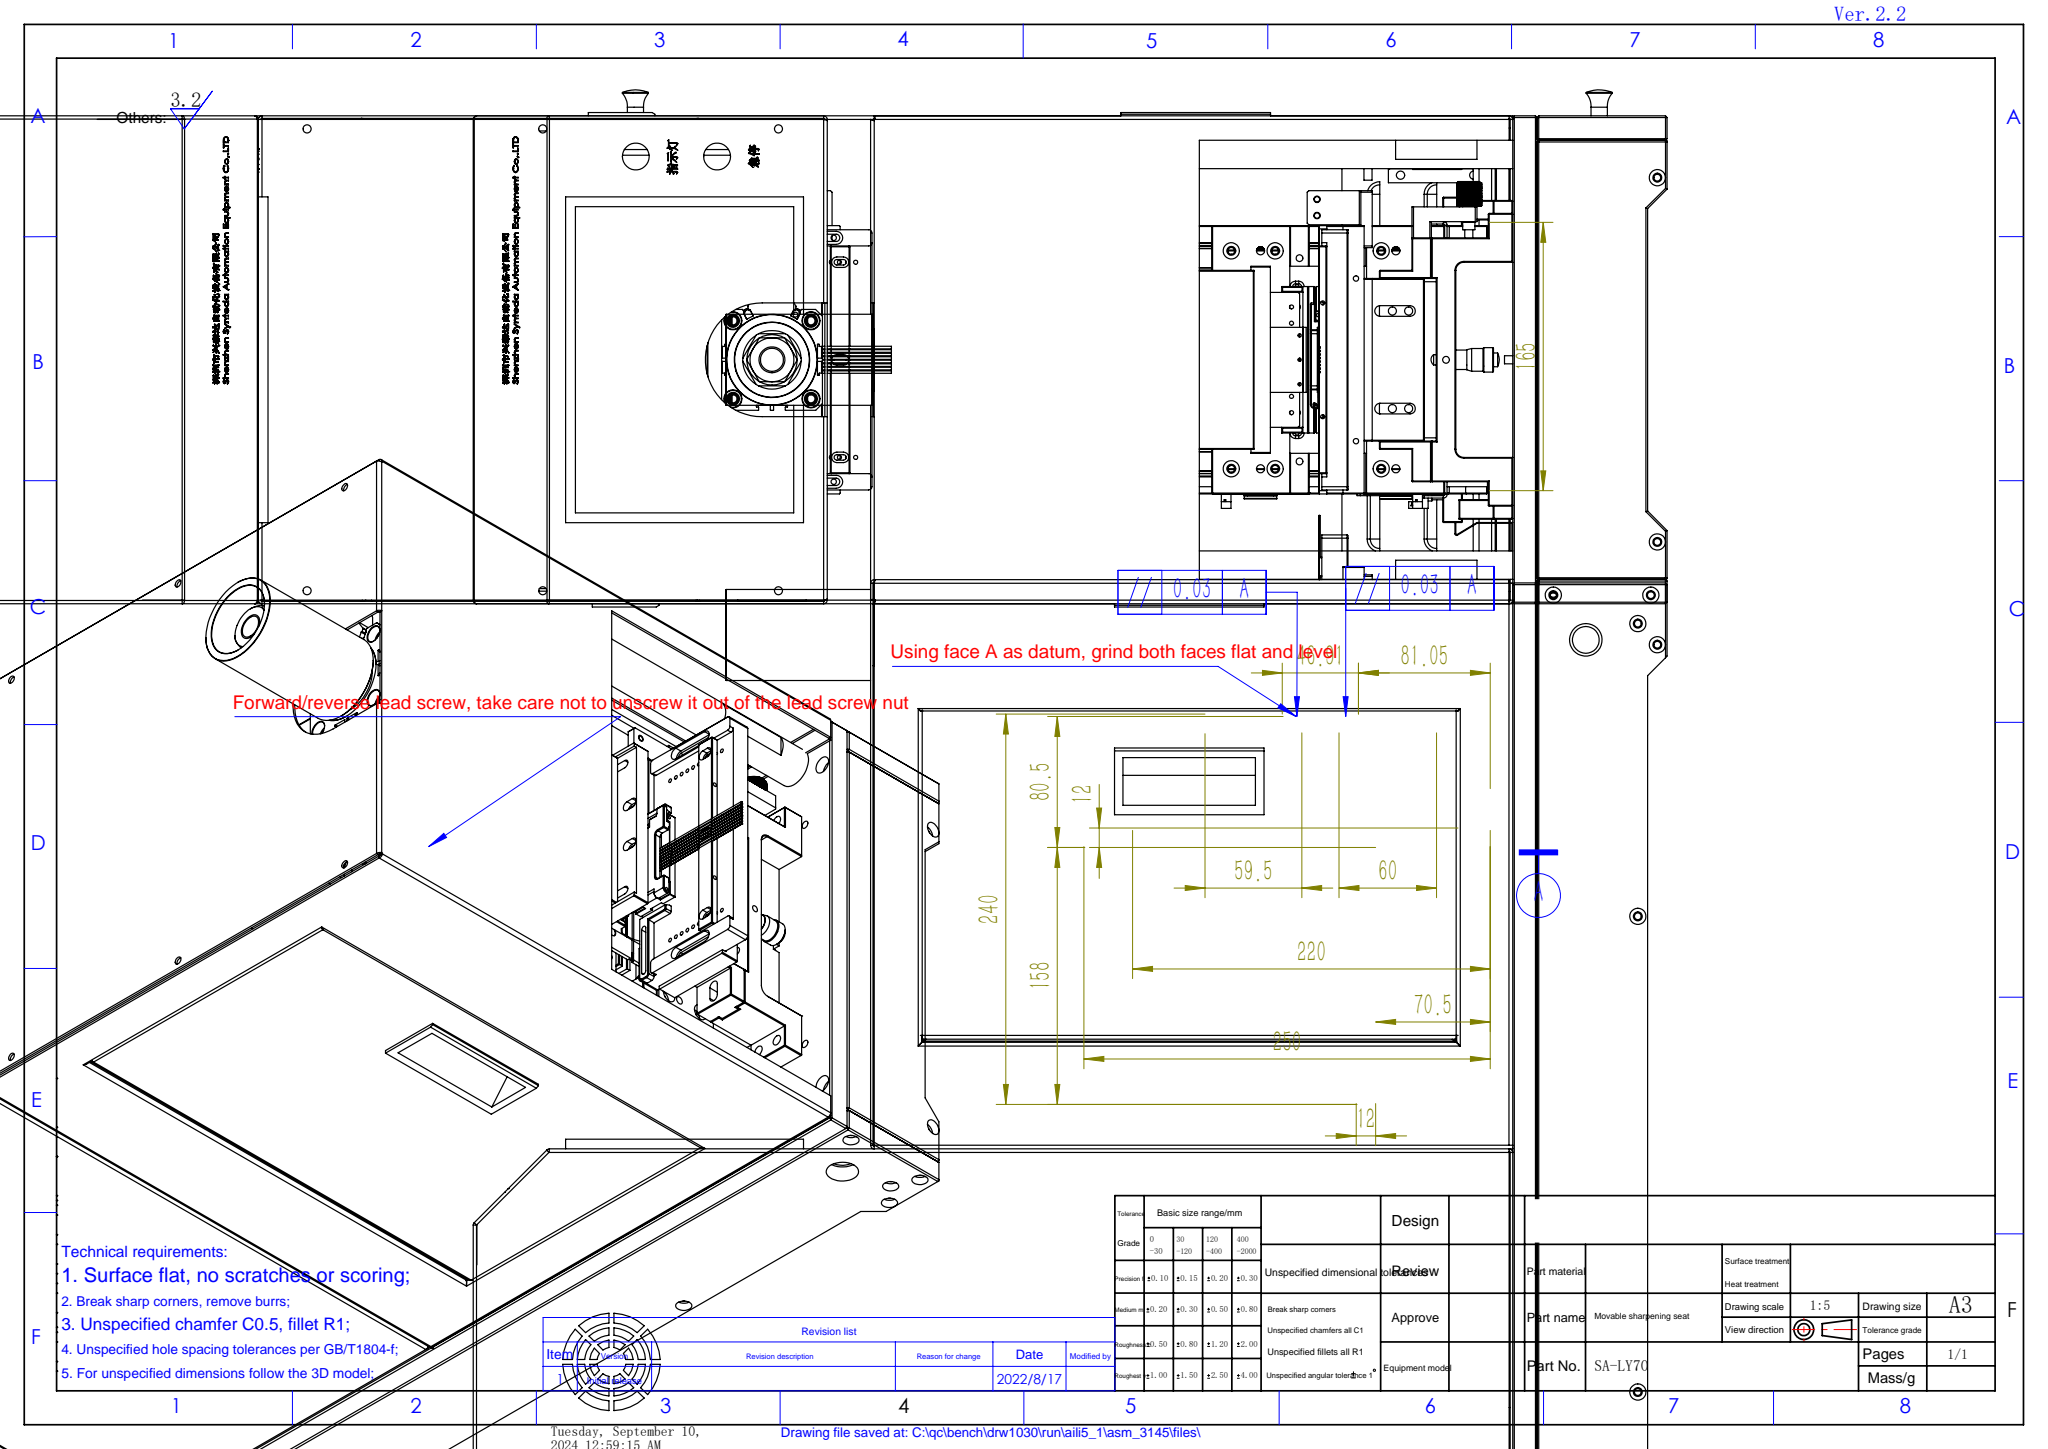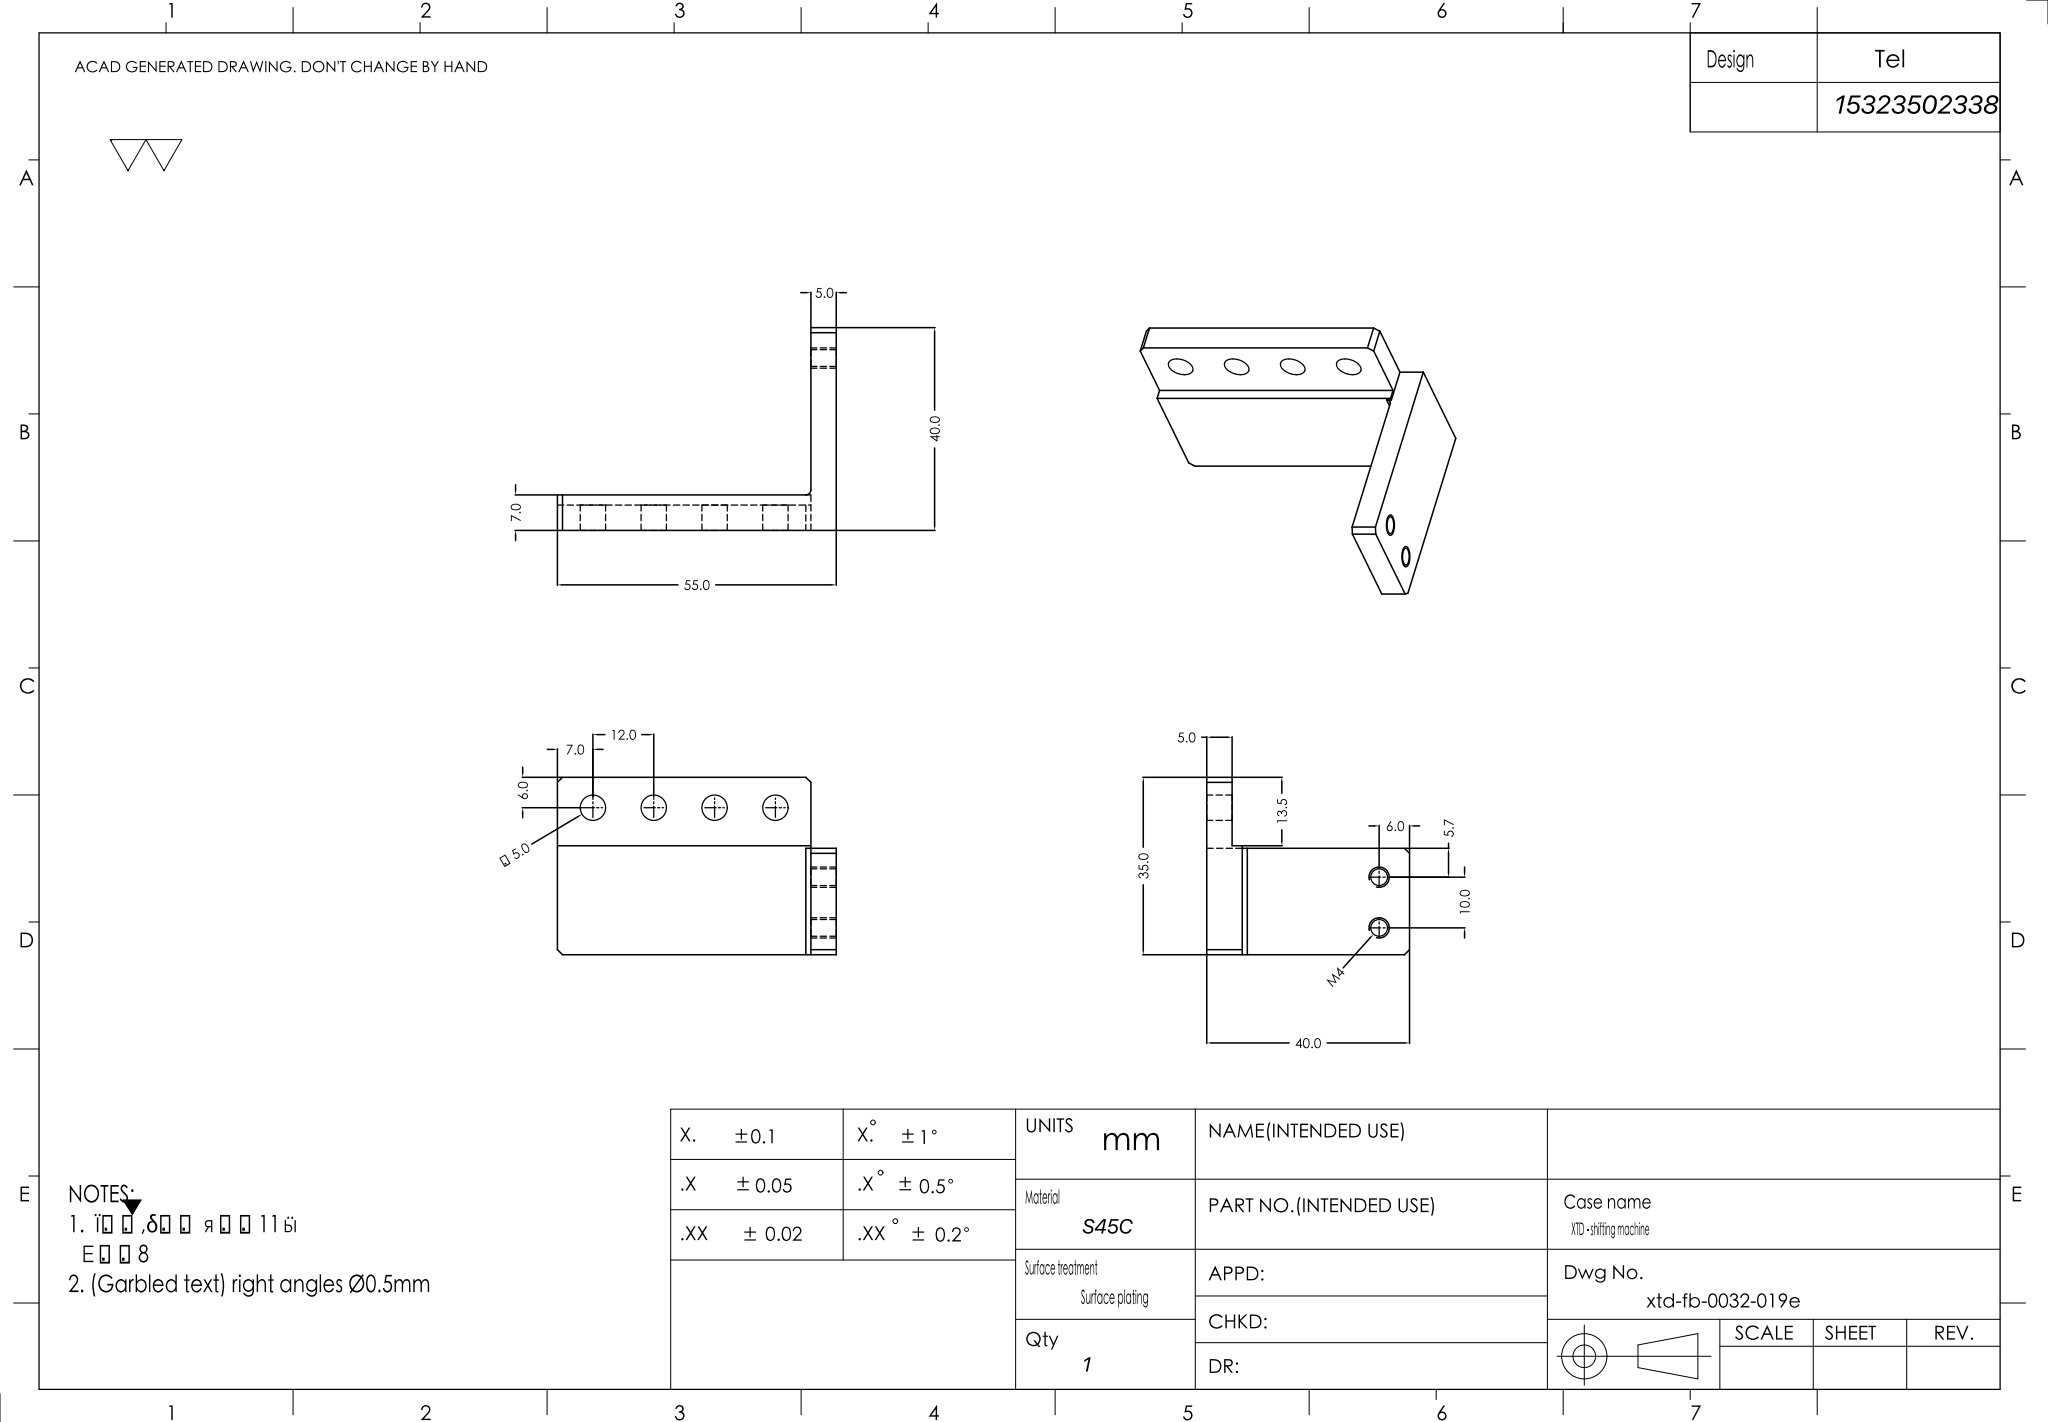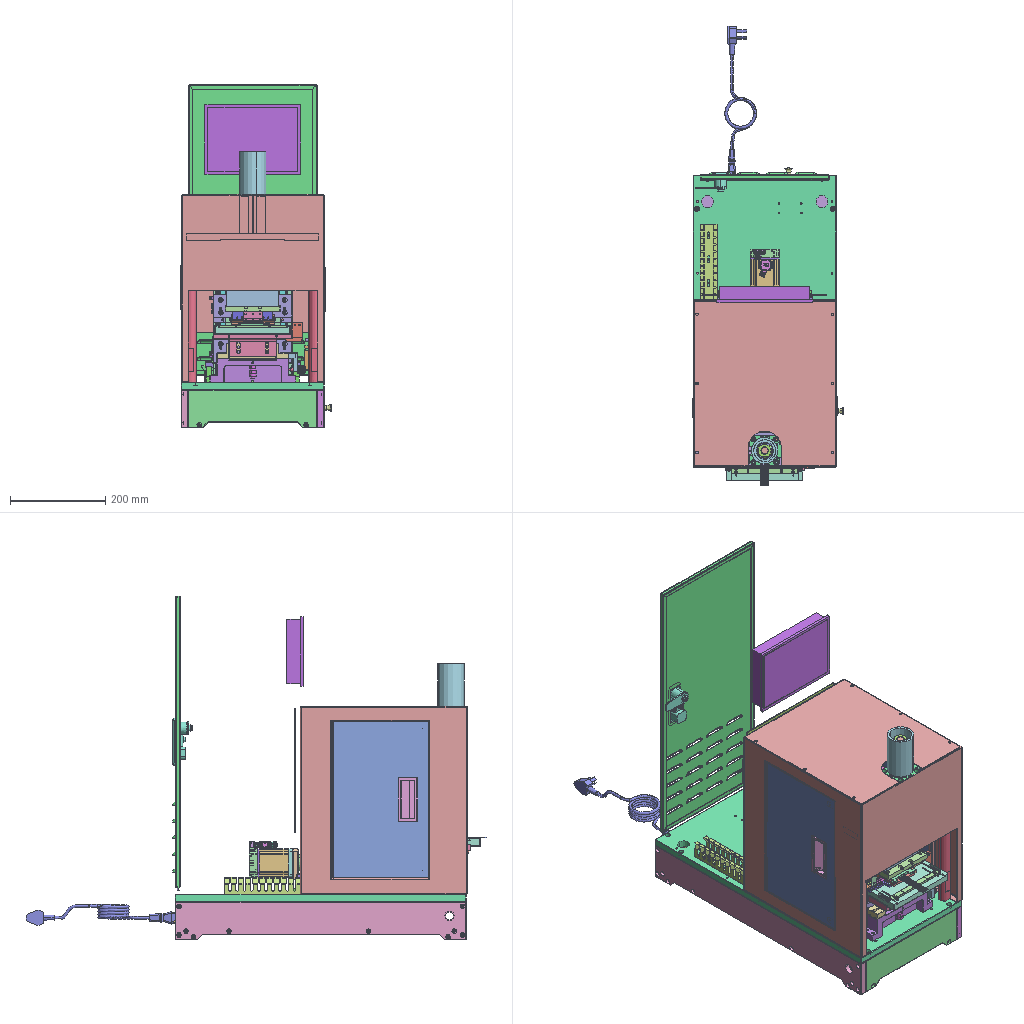Assembly | SolidWorks | 205 different items | 269 placed | box 318 x 965 x 720 mm
Parts list (item | name | quantity | parent item | size | volume | features):
1 | 0014 | x1 | - | - | - | -
2 | (subassembly) | x1 | in 17 | 12 x 43 x 43 mm | 7993 mm3 | -
3 | (subassembly) | x1 | in 17 | 110 x 14 x 40 mm | 34476 mm3 | -
4 | (subassembly) | x1 | - | 356.977 x 304 x 446.493 mm | 211386 mm3 | features ReferencePattern 2, InContextFeatHolder 1, MirrorCompFeat 1
5 | (subassembly) | x1 | - | 625.233 x 304 x 617.993 mm | 1412506 mm3 | features CompositeCurve 2, LocalLPattern 2, ReferencePattern 2
6 | (subassembly) | x1 | - | - | 1320917 mm3 | -
7 | (subassembly) | x1 | in 16 | 168.001 x 57 x 60 mm | 203187 mm3 | -
8 | (subassembly) | x1 | in 16 | 170.787 x 57.213 x 123 mm | 228547 mm3 | -
9 | (subassembly) | x1 | - | - | 1768279 mm3 | -
10 | (subassembly) | x1 | - | 316 x 923.1 x 130.5 mm | 5362274 mm3 | -
11 | (subassembly) | x1 | in 6 | 20 x 43 x 70 mm | 38437 mm3 | -
12 | (subassembly) | x1 | in 23 | - | - | -
13 | (subassembly) | x1 | in 6 | 35.5 x 43 x 70 mm | 61355 mm3 | -
14 | (subassembly) | x1 | in 17 | 150 x 40 x 36.569 mm | 33298 mm3 | -
15 | (subassembly) | x1 | in 6 | 150 x 39.987 x 40 mm | 33298 mm3 | -
16 | (subassembly) | x1 | - | - | 1570886 mm3 | -
17 | (subassembly) | x1 | - | - | 638711 mm3 | features CompositeCurve 1
18 | (subassembly) | x1 | in 16 | 40 x 213 x 40 mm | 59084 mm3 | -
19 | (subassembly) | x1 | in 16 | - | - | -
20 | (subassembly) | x1 | in 6 | 60 x 74.1 x 121 mm | 300230 mm3 | -
21 | (subassembly) | x1 | in 23 | - | - | -
22 | (subassembly) | x1 | in 12 | - | - | -
23 | (subassembly) | x1 | in 9 | 164.031 x 194.596 x 81.627 mm | 348427 mm3 | -
24 | (subassembly) | x1 | in 9 | 47 x 35.487 x 115 mm | 62999 mm3 | -
25 | (subassembly) | x2 | in 16 | 34 x 24 x 220 mm | 96136 mm3 | -
26 | (subassembly) | x2 | in 6 | 34 x 160 x 24 mm | 68410 mm3 | -
27 | (subassembly) | x2 | in 16, 17 | 35 x 52 x 52 mm | 28520 mm3 | -
28 | ATH-B0001 | x1 | - | - | - | -
29 | BML01-M6-L20 | x1 | - | - | - | -
30 | - | x1 | in 22 | - | - | features RefSurface 1
31 | - | x1 | in 17 | 70 x 72.5 x 10 mm | 34993 mm3 | features HoleWzd 3, Chamfer 2, Cut 2, Extrusion 1
32 | - | x1 | in 17 | 70 x 55 x 10 mm | 17124 mm3 | features Chamfer 2, Cut 2, HoleWzd 2, Extrusion 1, ICE 1
33 | - | x1 | in 17 | 70 x 55 x 10 mm | 20191 mm3 | features Chamfer 2, Cut 2, HoleWzd 2, Extrusion 1, ICE 1
34 | - | x1 | in 17 | 46 x 48 x 30 mm | 41518 mm3 | features HoleWzd 5, Chamfer 1, Cut 1, Extrusion 1, ICE 1
35 | - | x1 | in 17 | 76 x 68.5 x 10 mm | 24767 mm3 | features HoleWzd 4, Cut 3, Fillet 2, Chamfer 1, Extrusion 1, ICE 1
36 | - | x1 | in 17 | 60 x 76 x 14 mm | 29747 mm3 | features Cut 2, HoleWzd 2, Chamfer 1, Extrusion 1, Fillet 1, ICE 1
37 | - | x1 | in 17 | 120 x 35 x 10 mm | 16270 mm3 | features BaseBody 1
38 | - | x1 | in 10 | 235 x 120 x 40 mm | 81570 mm3 | features EdgeFlange 1, FlatPattern 1, HoleWzd 1, SMBaseFlange 1, SheetMetal 1
39 | - | x1 | in 10 | 40 x 100 x 120 mm | 42493 mm3 | features SMWeldBead 4, EdgeFlange 1, FlatPattern 1, HoleWzd 1, SMBaseFlange 1, SheetMetal 1
40 | - | x1 | in 8 | 170.003 x 76.5 x 17.003 mm | 25360 mm3 | features EdgeFlange 4, SMBaseFlange 2, Chamfer 1, FlatPattern 1, HoleWzd 1, SheetMetal 1
41 | - | x1 | in 22 | - | - | features RefSurface 1
42 | - | x2 | in 7, 8 | 20 x 36.964 x 3 mm | 709.216 mm3 | features EdgeFlange 2, Fillet 1, FlatPattern 1, HoleWzd 1, SMBaseFlange 1, SheetMetal 1
43 | - | x1 | in 16 | 20 x 36.464 x 3 mm | 699.216 mm3 | features EdgeFlange 2, Fillet 1, FlatPattern 1, HoleWzd 1, SMBaseFlange 1, SheetMetal 1
44 | - | x1 | in 17 | 20 x 36.5 x 25.2 mm | 1153 mm3 | features EdgeFlange 2, Fillet 1, FlatPattern 1, HoleWzd 1, SMBaseFlange 1, SheetMetal 1
45 | - | x1 | in 6 | 160 x 9 x 6 mm | 4968 mm3 | features BaseBody 1, Cut 1, HoleWzd 1, ICE 1, MoveFace 1
46 | - | x1 | in 17 | 105 x 9 x 6 mm | 3236 mm3 | features ICE 2, BaseBody 1, Cut 1, HoleWzd 1, MoveFace 1
47 | - | x1 | in 16 | 220 x 9 x 6 mm | 6858 mm3 | features BaseBody 1, Cut 1, HoleWzd 1, ICE 1, MoveFace 1
48 | - | x1 | - | 30 x 19 x 40 mm | 12917 mm3 | features ICE 2, Chamfer 1, Extrusion 1, HoleWzd 1
49 | - | x1 | - | 56 x 90 x 56 mm | 77215 mm3 | features Chamfer 1, Extrusion 1, ICE 1
50 | - | x1 | - | 35 x 35 x 2 mm | 1232 mm3 | features Extrusion 1
51 | - | x1 | in 9 | 170 x 62 x 71.5 mm | 267417 mm3 | features BaseBody 6
52 | - | x1 | in 22 | - | - | features RefSurface 1
53 | - | x1 | - | - | 2705 mm3 | features BaseBody 1
54 | - | x1 | in 9 | 8.4 x 18.475 x 16 mm | 1325 mm3 | features BaseBody 1
55 | - | x1 | in 9 | 17 x 19.6 x 45 mm | 6217 mm3 | features BaseBody 1
56 | - | x1 | in 23 | 55 x 50 x 165 mm | 141740 mm3 | features HoleWzd 5, ICE 2, Chamfer 1, Extrusion 1
57 | - | x1 | in 23 | - | - | features RefSurface 2, BaseBody 1
58 | - | x1 | in 24 | 7.5 x 20 x 90 mm | 7139 mm3 | features Chamfer 1, Extrusion 1, Fillet 1, HoleWzd 1, ICE 1
59 | - | x1 | in 23 | 140 x 12 x 5 mm | 7481 mm3 | features HoleWzd 2, Chamfer 1, Extrusion 1
60 | - | x2 | - | 115 x 2.5 x 23 mm | 5943 mm3 | features ICE 2, Extrusion 1, HoleWzd 1
61 | - | x1 | in 23 | 90 x 32.1 x 7 mm | 12925 mm3 | features Chamfer 3, Fillet 2, Extrusion 1, HoleWzd 1, ICE 1
62 | - | x1 | in 22 | - | - | features RefSurface 1
63 | - | x1 | in 24 | 40 x 7 x 21.5 mm | 5238 mm3 | features HoleWzd 2, Cut 1, Extrusion 1
64 | - | x1 | in 24 | 83 x 28 x 6 mm | 13498 mm3 | features HoleWzd 2, Chamfer 1, Extrusion 1
65 | - | x1 | in 24 | 40 x 7 x 6 mm | 1162 mm3 | features ICE 2, Extrusion 1
66 | - | x1 | in 24 | 115 x 12 x 37 mm | 35962 mm3 | features ICE 8, Cut 4, HoleWzd 4, Chamfer 1, Extrusion 1
67 | - | x2 | in 23 | 50 x 6 x 9 mm | 2366 mm3 | features Chamfer 1, Extrusion 1, HoleWzd 1
68 | - | x1 | in 23 | 90 x 10 x 5 mm | 4179 mm3 | features Chamfer 2, Extrusion 1, HoleWzd 1
69 | - | x1 | in 23 | 160 x 80 x 16 mm | 159297 mm3 | features ICE 8, HoleWzd 5, Chamfer 4, Extrusion 1, Fillet 1, LPattern 1
70 | - | x1 | in 23 | 47.5 x 23 x 5 mm | 1583 mm3 | features Fillet 2, Chamfer 1, Extrusion 1, HoleWzd 1, ICE 1
71 | - | x1 | in 23 | 47.5 x 23 x 5 mm | 1583 mm3 | features Fillet 2, Chamfer 1, Extrusion 1, HoleWzd 1, ICE 1
72 | - | x2 | in 2, 11 | 7 x 22 x 22 mm | 1819 mm3 | features BaseBody 1
73 | - | x1 | in 22 | - | - | features RefSurface 1
74 | - | x2 | in 14, 15 | 150 x 12 x 12 mm | 13946 mm3 | features BaseBody 1
75 | - | x2 | in 27 | 52 x 52 x 23 mm | 13989 mm3 | features BaseBody 1
76 | - | x2 | in 27 | 6.1 x 52 x 52 mm | 4618 mm3 | features BaseBody 1
77 | - | x2 | in 27 | 16 x 26 x 26 mm | 6727 mm3 | features BaseBody 1
78 | - | x4 | in 27 | 3 x 21 x 21 mm | 508.938 mm3 | features BaseBody 1
79 | - | x1 | in 2 | 43 x 43 x 12 mm | 6140 mm3 | features BaseBody 1
80 | - | x1 | in 11 | 70 x 43 x 20 mm | 36584 mm3 | features BaseBody 1
81 | - | x1 | in 13 | 24 x 43 x 70 mm | 47260 mm3 | features BaseBody 1
82 | - | x1 | in 13 | 8.1 x 34 x 34 mm | 4182 mm3 | features BaseBody 1
83 | - | x1 | in 13 | 16 x 26 x 26 mm | 6727 mm3 | features BaseBody 1
84 | - | x1 | in 22 | - | - | features RefSurface 1
85 | - | x2 | in 13 | 3 x 21 x 21 mm | 508.938 mm3 | features BaseBody 1
86 | - | x2 | in 27 | 19 x 19 x 8 mm | 1253 mm3 | features BaseBody 1
87 | - | x1 | in 13 | 19 x 19 x 8 mm | 1253 mm3 | features BaseBody 1
88 | - | x4 | in 27 | 14.4 x 14.4 x 5.5 mm | 457.404 mm3 | features BaseBody 1
89 | - | x2 | in 13 | 14.4 x 14.4 x 5.5 mm | 457.404 mm3 | features BaseBody 1
90 | - | x2 | in 2, 11 | 9.8 x 12 x 0.8 mm | 33.948 mm3 | features BaseBody 1
91 | - | x2 | in 10 | 16 x 22 x 16 mm | 1745 mm3 | features BaseBody 1
92 | - | x2 | in 17 | 10.392 x 19.5 x 9.5 mm | 848.731 mm3 | features BaseBody 1
93 | - | x1 | in 10 | 66.481 x 44.258 x 325.5 mm | 63656 mm3 | features MirrorStock 1
94 | - | x1 | in 10 | 35 x 35.5 x 353 mm | 17858 mm3 | features BaseBody 1, ICE 1
95 | - | x1 | in 22 | - | - | features RefSurface 1
96 | - | x2 | in 5 | 23.155 x 48.5 x 92 mm | 9910 mm3 | features BaseBody 1
97 | - | x1 | - | - | - | features RefSurface 1
98 | - | x1 | - | - | - | features RefSurface 1
99 | - | x1 | - | - | - | features RefSurface 1
100 | - | x1 | - | - | - | features RefSurface 1
101 | - | x1 | - | - | - | features RefSurface 1
102 | - | x3 | in 14, 15, 18 | 40 x 40 x 32 mm | 19352 mm3 | features BaseBody 1
103 | - | x1 | in 18 | 40 x 40 x 32 mm | 19352 mm3 | features BaseBody 1
104 | - | x1 | in 18 | 12 x 213 x 12 mm | 20380 mm3 | features BaseBody 1
105 | - | x1 | in 5 | 260 x 260 x 2 mm | 135000 mm3 | features Extrusion 1, Fillet 1, HoleWzd 1
106 | - | x1 | in 22 | - | - | features RefSurface 1
107 | - | x1 | in 10 | 51 x 50 x 32.3 mm | 28039 mm3 | features MirrorStock 1
108 | - | x1 | - | - | - | features RefSurface 1
109 | - | x1 | - | - | - | features RefSurface 1
110 | - | x1 | - | - | - | features RefSurface 1
111 | - | x1 | in 22 | - | - | features RefSurface 1
112 | - | x1 | in 22 | - | - | features RefSurface 1
113 | - | x1 | in 12 | - | - | features RefSurface 1
114 | - | x1 | in 22 | - | - | features RefSurface 1
115 | - | x1 | in 22 | - | - | features RefSurface 1
116 | - | x1 | in 22 | - | - | features RefSurface 1
117 | - | x1 | in 22 | - | - | features RefSurface 1
118 | - | x1 | in 22 | - | - | features RefSurface 1
119 | - | x1 | in 22 | - | - | features RefSurface 1
120 | - | x1 | in 22 | - | - | features RefSurface 1
121 | - | x1 | in 22 | - | - | features RefSurface 1
122 | - | x1 | in 22 | - | - | features RefSurface 1
123 | - | x1 | in 22 | - | - | features RefSurface 1
124 | - | x1 | in 22 | - | - | features RefSurface 1
125 | - | x1 | in 22 | - | - | features RefSurface 1
126 | - | x1 | in 22 | - | - | features RefSurface 1
127 | - | x1 | in 22 | - | - | features RefSurface 1
128 | - | x1 | in 22 | - | - | features RefSurface 1
129 | - | x1 | in 22 | - | - | features RefSurface 1
130 | - | x1 | in 17 | - | 141786 mm3 | features BaseBody 32
131 | - | x1 | - | - | - | features RefSurface 1
132 | - | x1 | - | - | - | features RefSurface 1
133 | - | x1 | - | - | - | features RefSurface 1
134 | - | x1 | - | - | - | features RefSurface 1
135 | - | x1 | in 22 | - | - | features RefSurface 1
136 | - | x1 | - | - | - | features RefSurface 1
137 | - | x4 | in 5 | 8 x 8 x 2 mm | 76.985 mm3 | features BaseBody 1
138 | - | x2 | in 6, 16 | 35 x 34 x 34 mm | 22881 mm3 | features BaseBody 1
139 | - | x1 | in 17 | 35 x 34 x 34 mm | 23327 mm3 | features BaseBody 1
140 | - | x9 | in 6, 16, 17 | 14.9 x 24.3 x 11.7 mm | 940.552 mm3 | features BaseBody 1
141 | - | x2 | in 26 | 15 x 12.5 x 160 mm | 25521 mm3 | features BaseBody 1
142 | - | x2 | in 25 | 15 x 12.5 x 220 mm | 34973 mm3 | features BaseBody 1, HoleWzd 1, MoveFace 1
143 | - | x1 | in 5 | 17.6 x 9 x 84 mm | 4996 mm3 | features BaseBody 2
144 | - | x1 | in 16 | 52 x 52 x 15 mm | 13321 mm3 | features BaseBody 1
145 | - | x4 | in 26 | 34 x 19.5 x 41.1 mm | 21445 mm3 | features BaseBody 1
146 | - | x1 | in 22 | - | - | features RefSurface 1
147 | - | x1 | in 5 | 395 x 300 x 350 mm | 661640 mm3 | features ICE 5, EdgeFlange 4, Cut 1, Fillet 1, FlatPattern 1, HoleWzd 1, LPattern 1, MirrorPattern 1, SMBaseFlange 1, SheetMetal 1
148 | - | x2 | in 5 | 333 x 204 x 10 mm | 124436 mm3 | features EdgeFlange 2, ICE 2, Cut 1, Fillet 1, FlatPattern 1, HoleWzd 1, SMBaseFlange 1, SheetMetal 1
149 | - | x4 | in 25 | 34 x 19.5 x 57.8 mm | 30582 mm3 | features BaseBody 1
150 | - | x1 | in 5 | 69.5 x 40 x 100 mm | 51575 mm3 | features BaseBody 1
151 | - | x1 | in 5 | - | - | -
152 | - | x1 | in 5 | 610.973 x 271.523 x 15.997 mm | 290304 mm3 | features EdgeFlange 2, Cut 1, FlatPattern 1, FormToolInstance 1, LPattern 1, SMBaseFlange 1, SheetMetal 1
153 | - | x1 | in 3 | 40 x 10.6 x 46.1 mm | 13496 mm3 | features BaseBody 1
154 | - | x1 | in 3 | 24 x 8.5 x 110 mm | 20980 mm3 | features BaseBody 1
155 | - | x1 | in 9 | 42 x 15 x 15 mm | 4392 mm3 | features BaseBody 1
156 | - | x1 | in 19 | - | - | features BaseBody 21, RefSurface 11
157 | - | x1 | in 22 | - | - | features RefSurface 1
158 | - | x1 | in 20 | 60 x 74.1 x 121 mm | 300230 mm3 | features BaseBody 24
159 | - | x1 | - | 200.3 x 146.3 x 34 mm | 870408 mm3 | features ICE 2, Extrusion 1
160 | - | x1 | - | - | - | features RefSurface 1
161 | - | x2 | in 9 | 37.5 x 47.5 x 18 mm | 8206 mm3 | features BaseBody 1
162 | - | x2 | in 19, 20 | - | - | -
163 | - | x2 | in 19, 20 | - | - | -
164 | - | x2 | in 19, 20 | - | - | -
165 | - | x1 | in 9 | 296 x 62 x 15 mm | 226499 mm3 | features HoleWzd 3, Chamfer 2, Cut 2, Extrusion 1
166 | - | x1 | in 9 | 135 x 100 x 27 mm | 173554 mm3 | features HoleWzd 2, ICE 2, Chamfer 1, Cut 1, Extrusion 1, Fillet 1
167 | - | x1 | in 9 | 110 x 90 x 15 mm | 144771 mm3 | features Cut 2, Chamfer 1, Extrusion 1, HoleWzd 1
168 | - | x1 | in 22 | - | - | features RefSurface 1
169 | - | x2 | in 9 | 10 x 100 x 20 mm | 18869 mm3 | features Chamfer 1, Extrusion 1, HoleWzd 1
170 | - | x2 | in 9 | 25 x 25 x 300 mm | 142022 mm3 | features Chamfer 1, Extrusion 1, HoleWzd 1, ICE 1, MirrorPattern 1
171 | - | x1 | in 9 | 180 x 30 x 50 mm | 139054 mm3 | features Cut 4, HoleWzd 4, ICE 2, Chamfer 1, Extrusion 1, Fillet 1
172 | - | x1 | in 9 | 150 x 35 x 30 mm | 55419 mm3 | features ICE 4, Chamfer 1, Extrusion 1, HoleWzd 1, LPattern 1
173 | - | x1 | in 10 | 270 x 80 x 15 mm | 285008 mm3 | features HoleWzd 3, Chamfer 2, Cut 1, Extrusion 1, MirrorPattern 1
174 | - | x1 | in 10 | 270 x 80 x 15 mm | 180697 mm3 | features Cut 4, HoleWzd 4, Chamfer 2, ICE 2, Extrusion 1, Fillet 1, MirrorPattern 1
175 | - | x1 | in 10 | 200 x 270 x 12 mm | 548140 mm3 | features Chamfer 2, HoleWzd 2, Cut 1, Extrusion 1, MirrorPattern 1
176 | - | x1 | in 10 | 105 x 270 x 12 mm | 306899 mm3 | features Chamfer 2, HoleWzd 2, Cut 1, Extrusion 1, MirrorPattern 1
177 | - | x1 | in 10 | 610 x 80 x 15 mm | 627969 mm3 | features HoleWzd 4, Cut 3, Chamfer 2, Extrusion 1
178 | - | x1 | in 10 | 610 x 80 x 15 mm | 549911 mm3 | features Cut 5, HoleWzd 3, Chamfer 2, Extrusion 1, ICE 1
179 | - | x1 | in 22 | - | - | features RefSurface 1
180 | - | x4 | in 10 | 30 x 30 x 12 mm | 7848 mm3 | features HoleWzd 3, Chamfer 2, Extrusion 1
181 | - | x1 | in 10 | 610 x 300 x 15 mm | 2595255 mm3 | features HoleWzd 9, Cut 3, Chamfer 1, Extrusion 1, Fillet 1, LPattern 1
182 | - | x2 | in 6 | 215 x 33 x 12 mm | 75834 mm3 | features ICE 3, HoleWzd 2, Chamfer 1, Extrusion 1
183 | - | x1 | in 6 | 200 x 187 x 12 mm | 387596 mm3 | features HoleWzd 7, Cut 4, Chamfer 1, Extrusion 1
184 | - | x2 | in 6 | 160 x 25 x 19 mm | 67166 mm3 | features HoleWzd 3, ICE 2, Chamfer 1, Cut 1, Extrusion 1
185 | - | x1 | in 16 | 160 x 165 x 12 mm | 211716 mm3 | features HoleWzd 8, Cut 4, Chamfer 2, ICE 2, LPattern 2, Extrusion 1
186 | - | x1 | in 16 | 40 x 20 x 10 mm | 7263 mm3 | features Chamfer 2, HoleWzd 2, Extrusion 1
187 | - | x1 | in 6 | 95 x 65 x 12 mm | 46532 mm3 | features Chamfer 2, HoleWzd 2, Cut 1, Extrusion 1
188 | - | x2 | in 16 | 158 x 167.5 x 12 mm | 69045 mm3 | features HoleWzd 2, ICE 2, Chamfer 1, Cut 1, Extrusion 1, Fillet 1
189 | - | x1 | in 16 | 46 x 36 x 22 mm | 23549 mm3 | features HoleWzd 2, Chamfer 1, Cut 1, Extrusion 1
190 | - | x1 | in 22 | - | - | features RefSurface 1
191 | - | x1 | in 16 | 165 x 250 x 12 mm | 353527 mm3 | features HoleWzd 8, Cut 5, ICE 2, Chamfer 1, Extrusion 1
192 | - | x2 | in 16 | 220 x 21 x 19 mm | 76090 mm3 | features HoleWzd 4, ICE 2, Chamfer 1, Cut 1, Extrusion 1
193 | - | x2 | in 16 | 70 x 48 x 10 mm | 15539 mm3 | features Chamfer 2, Cut 2, HoleWzd 2, Extrusion 1, ICE 1
194 | - | x2 | in 16 | 50 x 34 x 30 mm | 33922 mm3 | features HoleWzd 3, Chamfer 1, Cut 1, Extrusion 1, ICE 1, MirrorPattern 1
195 | - | x1 | in 16 | 65 x 69 x 10 mm | 21766 mm3 | features HoleWzd 3, Cut 2, Chamfer 1, Extrusion 1
196 | - | x2 | in 7, 8 | 165 x 60 x 20 mm | 97648 mm3 | features HoleWzd 8, Cut 4, Chamfer 2, ICE 2, MirrorPattern 2, Extrusion 1, Fillet 1
197 | - | x2 | in 7, 8 | 60 x 165 x 14 mm | 104829 mm3 | features BaseBody 1
198 | - | x1 | in 17 | 70 x 50 x 10 mm | 29582 mm3 | features HoleWzd 3, Chamfer 1, Cut 1, Extrusion 1
199 | - | x1 | in 17 | 120 x 38 x 10 mm | 40489 mm3 | features Chamfer 2, HoleWzd 2, Extrusion 1
200 | - | x1 | in 17 | 70 x 169.5 x 10 mm | 105739 mm3 | features HoleWzd 6, Cut 4, Chamfer 1, Extrusion 1, ICE 1
201 | - | x1 | in 12 | - | - | features RefSurface 1
202 | LYE Electrical Cabinet 01 | x1 | - | - | - | -
203 | LYE Electrical Cabinet 02 | x1 | - | - | - | -
204 | LY Electrical Cabinet 01 | x1 | - | - | - | -
205 | LY Electrical Cabinet 02 | x1 | - | - | - | -
Mates (type | each side: item.copy, entity, surface, feature), first 278 of 404 lines:
In the top assembly
Parallel | 178.1 face plane Cut-Extrude 2 | assembly face
Concentric | 181.1 face cylinder Cut-Extrude 4 | 170.1 face cylinder Boss-Extrude 1
Coincident | 181.1 face plane Cut-Extrude 4 | 170.1 face plane Boss-Extrude 1
Concentric | 181.1 face cylinder Cut-Extrude 4 | 170.2 face cylinder Boss-Extrude 1
Coincident | 147.1 face plane Edge-Flange 2 | 94.1 face plane  Import 1
Concentric | assembly face | 53.1 face cylinder  Import 1
Coincident | assembly face | 48.1 face plane Boss-Extrude 1 | 2 times
Coincident | assembly face | 48.1 face plane Boss-Extrude 2
DistanceDim | 53.1 face plane  Import 1 | assembly face
Coincident | 145.1 face plane  Import 1 | 185.1 face plane Cut-Extrude 2
Concentric | 145.1 face cylinder  Import 1 | 185.1 face cylinder M4 Hex Socket Screw Counterbore Hole 2 | 2 times
Coincident | 102.1 face plane  Import 1 | 189.1 face plane Boss-Extrude 1
Coincident | 198.1 face plane Boss-Extrude 1 | 185.1 face plane Cut-Extrude 3
Width | 198.1 face plane Boss-Extrude 1 | 198.1 face plane Boss-Extrude 1 | 185.1 face plane Cut-Extrude 3 | 185.1 face plane Cut-Extrude 3
DistanceDim | 198.1 face plane Boss-Extrude 1 | 186.1 face plane Boss-Extrude 1
Concentric | 51.1 face cylinder _SDAJS-50x40_40b-1-solid1 | 49.1 face cylinder Boss-Extrude 1
Coincident | 51.1 face plane _SDAJS-50x40_40b-1-solid1 | 49.1 face plane Boss-Extrude 1
Coincident | 49.1 edge | 50.1 face plane Boss-Extrude 1
Concentric | 51.1 face cylinder _SDAJS-50x401040_r-1-solid1 | 50.1 face cylinder Boss-Extrude 1
DistanceDim | 182.1 face plane Boss-Extrude 2 | 94.1 face plane  Import 1
Coincident | 197.1 face plane  Import 1 | 60.1 face plane Boss-Extrude 1
Slot | 60.1 face plane M3 Hex Socket Countersunk Screw Countersink Hole 1 | 197.1 face cylinder  Import 1
Slot | 197.1 face cylinder  Import 1 | 60.1 face plane M3 Hex Socket Countersunk Screw Countersink Hole 1
Coincident | 197.2 face plane  Import 1 | 60.2 face plane Boss-Extrude 1
Slot | 60.2 face plane M3 Hex Socket Countersunk Screw Countersink Hole 1 | 197.2 face cylinder  Import 1
Parallel | 197.2 face plane  Import 1 | 60.2 face plane Boss-Extrude 1
Coincident | 182.2 face plane Boss-Extrude 1 | 181.1 face plane Boss-Extrude 1
Parallel | 182.2 face cylinder Ø6.5 (6.5) DiameterHole 1 | 181.1 face cylinder M6 Tapped Hole 1
Width | 181.1 face plane Boss-Extrude 1 | 181.1 face plane Boss-Extrude 1 | 182.2 face plane Boss-Extrude 1 | 182.1 face plane Boss-Extrude 1
Width | 196.1 face plane Boss-Extrude 1 | 196.2 face plane Boss-Extrude 1 | 36.1 face plane Boss-Extrude 1 | 36.1 face plane Boss-Extrude 1
LimitDistanceDim | 185.1 face plane Boss-Extrude 1 | 184.1 face plane Boss-Extrude 1
In subassembly 6
Parallel | 187.1 face plane Boss-Extrude 1 | 183.1 face plane Boss-Extrude 1
Concentric | 187.1 face cylinder Ø6.5 (6.5) DiameterHole 1 | 183.1 face cylinder M6 Tapped Hole 1
Coincident | 187.1 face plane Boss-Extrude 1 | 183.1 face plane Cut-Extrude 5
Width | 182.3 face plane Boss-Extrude 1 | 182.3 face plane Boss-Extrude 1 | 183.1 face plane Cut-Extrude 4 | 183.1 face plane Cut-Extrude 4
Coincident | 182.3 face plane Boss-Extrude 1 | 183.1 face plane Cut-Extrude 4
Coincident | 182.3 face plane Boss-Extrude 1 | 183.1 face plane Boss-Extrude 1
Width | 182.4 face plane Boss-Extrude 1 | 182.4 face plane Boss-Extrude 1 | 183.1 face plane Cut-Extrude 4 | 183.1 face plane Cut-Extrude 4
Coincident | 183.1 face plane Cut-Extrude 4 | 182.4 face plane Boss-Extrude 1
Coincident | 183.1 face plane Boss-Extrude 1 | 182.4 face plane Boss-Extrude 1
Coincident | 184.2 face plane Boss-Extrude 1 | 183.1 face plane Cut-Extrude 6
Coincident | 184.3 face plane Boss-Extrude 1 | 183.1 face plane Cut-Extrude 6
Concentric | 184.2 face cylinder M6 Hex Socket Screw Counterbore Hole 1 | 183.1 face cylinder M6 Tapped Hole 2
Concentric | 184.3 face cylinder M6 Hex Socket Screw Counterbore Hole 1 | 183.1 face cylinder M6 Tapped Hole 2 | 2 times
Coincident | 184.2 face plane Boss-Extrude 1 | 45.1 face plane  Import 1
Concentric | 184.2 face cylinder M3 Tapped Hole 1 | 45.1 face cylinder M3 Hex Socket Screw Counterbore Hole 1 | 2 times
Coincident | 45.1 face plane  Import 1 | 140.1 face plane Imported1
Coincident | 45.1 face plane  Import 1 | 140.2 face plane Imported1
Coincident | 140.1 face plane Imported1 | 140.2 face plane Imported1
Coincident | 187.1 face plane Boss-Extrude 1 | 158.1 face plane MS1H1-40B30CB-A331Z_21-1-solid1
Concentric | 187.1 face cylinder Cut-Extrude 1 | 158.1 face cylinder MS1H1-40B30CB-A331Z_21-1-solid1
Parallel | 187.1 face plane Boss-Extrude 1 | 158.1 face plane MS1H1-40B30CB-A331Z_21-1-solid1
Coincident | 184.2 face plane Cut-Extrude 1 | 141.1 face plane  Import 1
Concentric | 184.2 face cylinder M4 Tapped Hole 1 | 141.1 face cylinder  Import 1 | 2 times
Concentric | 183.1 face cylinder M6 Tapped Hole 2 | 184.2 face cylinder M6 Hex Socket Screw Counterbore Hole 1
Concentric | 74.1 face cylinder  Import 1 | 89.1 face cylinder  Import 1
Concentric | 74.1 face cylinder  Import 1 | 72.1 face cylinder  Import 1
Coincident | 74.1 face plane  Import 1 | 72.1 face plane  Import 1
Parallel | 81.1 face plane  Import 1 | 6.1 face
Coincident | 6.1 face | 89.1 face plane  Import 1
Coincident | 81.1 face plane  Import 1 | 80.1 face plane  Import 1
Concentric | 74.1 face cylinder  Import 1 | 138.1 face cylinder  Import 1
Coincident | 74.1 face plane  Import 1 | 138.1 face plane  Import 1
Parallel | 183.1 face plane Cut-Extrude 3 | 81.1 face plane  Import 1
Coincident | 183.1 face plane Cut-Extrude 3 | 81.1 face plane  Import 1
Width | 81.1 face plane  Import 1 | 81.1 face plane  Import 1 | 183.1 face plane Cut-Extrude 3 | 183.1 face plane Cut-Extrude 3
Coincident | 184.3 face plane Cut-Extrude 1 | 141.2 face plane  Import 1 | 2 times
Concentric | 184.3 face cylinder M4 Tapped Hole 1 | 141.2 face cylinder  Import 1
Width | 140.2 face plane Imported1 | 140.2 face plane Imported1 | 45.1 face plane  Import 1 | 45.1 face plane  Import 1
Coincident | 140.1 face plane Imported1 | 140.3 face plane Imported1 | 2 times
Coincident | 183.1 face plane Cut-Extrude 3 | 80.1 face plane  Import 1
Parallel | 183.1 face cylinder M8 Tapped Hole 1 | 80.1 face cylinder  Import 1
Concentric | 183.1 face cylinder M8 Tapped Hole 1 | 80.1 face cylinder  Import 1
Coincident | 74.1 face plane  Import 1 | 89.1 face plane  Import 1
Coincident | 145.2 face plane  Import 1 | 145.3 face plane  Import 1
Coincident | 145.4 face plane  Import 1 | 145.5 face plane  Import 1
Parallel | 102.2 face plane  Import 1 | 80.1 face plane  Import 1
In subassembly 26
DistanceDim | 145.6 face plane  Import 1 | 141.3 face plane  Import 1 | 2 times
Coincident | 145.7 face plane  Import 1 | 145.6 face plane  Import 1 | 2 times
In subassembly 15
Concentric | 74.2 face cylinder  Import 1 | 102.3 face cylinder  Import 1
In subassembly 5
Width | 150.1 face plane  Import 1 | 150.1 face plane  Import 1 | 152.1 face plane Cut-Extrude 1 | 152.1 face plane Cut-Extrude 1 | 2 times
Coincident | 152.1 face plane Base-Flange 1 | 150.1 face plane  Import 1
Coincident | 147.2 face plane Edge-Flange 4 | 148.1 face plane Edge-Flange 2
DistanceDim | 148.1 face plane Edge-Flange 1 | 147.2 face plane Edge-Flange 3
Width | 147.2 face plane Edge-Flange 3 | 147.2 face plane Edge-Flange 3 | 148.1 face plane Edge-Flange 1 | 148.1 face plane Edge-Flange 1
Width | 96.1 face plane  Import 1 | 96.1 face plane  Import 1 | 148.1 face plane Cut-Extrude 1 | 148.1 face plane Cut-Extrude 1
Width | 148.1 face plane Cut-Extrude 1 | 148.1 face plane Cut-Extrude 1 | 96.1 face plane  Import 1 | 96.1 face plane  Import 1
Coincident | 148.1 face plane Base-Flange 1 | 96.1 face plane  Import 1
Width | 147.2 face plane Edge-Flange 3 | 147.2 face plane Edge-Flange 3 | 148.2 face plane Edge-Flange 1 | 148.2 face plane Edge-Flange 1
Coincident | 147.2 face plane Edge-Flange 4 | 148.2 face plane Edge-Flange 2
DistanceDim | 148.2 face plane Edge-Flange 1 | 147.2 face plane Edge-Flange 3
Width | 148.2 face plane Cut-Extrude 1 | 148.2 face plane Cut-Extrude 1 | 96.2 face plane  Import 1 | 96.2 face plane  Import 1
Width | 96.2 face plane  Import 1 | 96.2 face plane  Import 1 | 148.2 face plane Cut-Extrude 1 | 148.2 face plane Cut-Extrude 1
Coincident | 148.2 face plane Base-Flange 1 | 96.2 face plane  Import 1
Coincident | 152.1 face plane Base-Flange 1 | 143.1 face plane _HFG86-17-001-1-solid1
Coincident | 152.1 edge | 143.1 face plane _HFG86-17-001-1-solid1
Parallel | 152.1 face plane Edge-Flange 1 | 143.1 face plane _HFG86-17-001-1-solid1
Coincident | 148.1 face plane Cut-Extrude 2 | 137.1 face plane  Import 1
Concentric | 137.1 face cylinder  Import 1 | 148.1 face cylinder M3 Tapped Hole 2
Coincident | 148.2 face plane Cut-Extrude 2 | 137.2 edge
Concentric | 148.2 face cylinder Cut-Extrude 2 | 137.2 edge
In subassembly 17
Coincident | 35.1 face plane Cut-Extrude 3 | 34.1 face plane Boss-Extrude 1
Width | 35.1 face plane Cut-Extrude 4 | 35.1 face plane Cut-Extrude 4 | 36.2 face plane Boss-Extrude 1 | 36.2 face plane Boss-Extrude 1
Coincident | 35.1 face plane Cut-Extrude 4 | 36.2 face plane Boss-Extrude 1
Width | 35.1 face plane Boss-Extrude 1 | 35.1 face plane Boss-Extrude 1 | 36.2 face plane Boss-Extrude 1 | 36.2 face plane Boss-Extrude 1
Coincident | 36.2 face plane Cut-Extrude 1 | 37.1 face plane  Import 1
Width | 36.2 face plane Boss-Extrude 1 | 36.2 face plane Boss-Extrude 1 | 37.1 face plane  Import 1 | 37.1 face plane  Import 1 | 2 times
Width | 200.1 face plane Cut-Extrude 2 | 200.1 face plane Cut-Extrude 2 | 33.1 face plane Boss-Extrude 1 | 33.1 face plane Boss-Extrude 1
Coincident | 200.1 face plane Cut-Extrude 1 | 33.1 face plane Boss-Extrude 1
Coincident | 200.1 face plane Boss-Extrude 1 | 199.1 face plane Boss-Extrude 1
Width | 46.1 face plane  Import 1 | 46.1 face plane  Import 1 | 200.1 face plane Boss-Extrude 1 | 200.1 face plane Boss-Extrude 1
Coincident | 200.1 face plane Boss-Extrude 1 | 46.1 face plane  Import 1
Coincident | 200.1 face plane Boss-Extrude 1 | 31.1 face plane Cut-Extrude 1
Concentric | 200.1 face cylinder M5 Tapped Hole 2 | 31.1 face cylinder M5 Hex Socket Screw Counterbore Hole 1 | 2 times
Width | 200.1 face plane Boss-Extrude 1 | 200.1 face plane Boss-Extrude 1 | 79.1 face plane  Import 1 | 79.1 face plane  Import 1
Parallel | 75.1 face plane  Import 1 | 79.1 face plane  Import 1
Concentric | 79.1 face cylinder  Import 1 | 33.1 face cylinder Cut-Extrude 2
Parallel | 79.1 face plane  Import 1 | 33.1 face plane Boss-Extrude 1
Coincident | 79.1 face plane  Import 1 | 33.1 face plane Boss-Extrude 1
Coincident | 34.1 face plane Boss-Extrude 1 | 44.1 face plane Base-Flange 1
Coincident | 31.1 face plane Boss-Extrude 1 | 130.1 face plane 57CME26_25-1-solid1
Concentric | 31.1 face cylinder Cut-Extrude 2 | 130.1 face cylinder 57CME26_25-1-solid1
Concentric | 31.1 face cylinder M4 Tapped Hole 1 | 130.1 face cylinder 57CME26_25-1-solid1
Concentric | 35.1 face cylinder M5 Hex Socket Screw Counterbore Hole 2 | 34.1 face cylinder M5 Tapped Hole 1 | 2 times
Concentric | 200.1 face cylinder M5 Hex Socket Screw Counterbore Hole 1 | 199.1 face cylinder M5 Tapped Hole 2 | 2 times
Width | 34.1 face plane Cut-Extrude 1 | 34.1 face plane Cut-Extrude 1 | 153.1 face plane  Import 1 | 153.1 face plane  Import 1
Coincident | 34.1 face plane Cut-Extrude 1 | 153.1 face plane  Import 1
Width | 153.1 face plane  Import 1 | 153.1 face plane  Import 1 | 34.1 face plane Boss-Extrude 1 | 34.1 face plane Boss-Extrude 1
Width | 154.1 face plane  Import 1 | 154.1 face plane  Import 1 | 200.1 face plane Cut-Extrude 1 | 200.1 face plane Cut-Extrude 1
Coincident | 200.1 face plane Cut-Extrude 1 | 154.1 face plane  Import 1
Concentric | 200.1 face cylinder M4 Tapped Hole 1 | 154.1 face cylinder  Import 1
Coincident | 46.1 face plane  Import 1 | 140.1 face plane Imported1
Width | 46.1 face plane  Import 1 | 46.1 face plane  Import 1 | 140.1 face cylinder Imported1
Parallel | 46.1 face plane  Import 1 | 140.1 face plane Imported1
Concentric | 34.1 face cylinder M3 Tapped Hole 2 | 44.1 face cylinder Ø3.5 (3.5) Diameter Slot 1 | 2 times
Concentric | 72.2 face cylinder  Import 1 | 74.3 face cylinder  Import 1
Coincident | 72.2 face plane  Import 1 | 74.3 face plane  Import 1
Parallel | 200.1 face plane Boss-Extrude 1 | 102.4 face plane  Import 1
Coincident | 34.1 face plane Boss-Extrude 1 | 102.4 face plane  Import 1
Coincident | 88.1 face plane  Import 1 | 74.3 face plane  Import 1
Concentric | 75.1 face cylinder  Import 1 | 74.3 face cylinder  Import 1
Coincident | 75.1 face plane  Import 1 | 32.1 face plane Boss-Extrude 1
Concentric | 200.1 face cylinder M5 Tapped Hole 1 | 32.1 face cylinder Ø5.5 (5.5) DiameterHole 1
Coincident | 200.1 face plane Cut-Extrude 1 | 32.1 face plane Boss-Extrude 1
Coincident | 46.1 face plane  Import 1 | 140.2 face plane Imported1
Coincident | 46.1 face plane  Import 1 | 140.3 face plane Imported1
Coincident | 140.1 face plane Imported1 | 140.2 face plane Imported1
Coincident | 140.2 face plane Imported1 | 140.3 face plane Imported1
Coincident | 200.1 face plane Boss-Extrude 1 | 198.2 face plane Cut-Extrude 1
Concentric | 200.1 face cylinder M5 Tapped Hole 3 | 198.2 face cylinder M5 Hex Socket Screw Counterbore Hole 1
Coincident | 200.1 face plane Boss-Extrude 1 | 198.2 face plane Boss-Extrude 1
Concentric | 92.1 face cylinder PC4M5 | 37.1 edge
Coincident | 37.1 face plane  Import 1 | 92.1 face plane PC4M5
Concentric | 92.2 face cylinder PC4M5 | 37.1 face cylinder  Import 1
Coincident | 37.1 face plane  Import 1 | 92.2 face plane PC4M5
Concentric | 130.1 face cylinder 57CME26_12-1-solid1 | 139.1 face cylinder DBJ52-D34-d8-e8
Coincident | 74.3 face plane  Import 1 | 139.1 face plane DBJ52-D34-d8-e8
Concentric | 200.1 face cylinder M3 Tapped Hole 1 | 46.1 face cylinder M3 Hex Socket Screw Counterbore Hole 1
In subassembly 14
Concentric | 74.2 face cylinder  Import 1 | 102.3 face cylinder  Import 1
In subassembly 3
Coincident | 153.2 face plane  Import 1 | 154.2 face plane  Import 1
Width | 153.2 face plane  Import 1 | 153.2 face plane  Import 1 | 154.2 face plane  Import 1 | 154.2 face plane  Import 1
Coincident | 154.2 face plane  Import 1 | 3.1 plane | 2 times
In subassembly 10
Concentric | 38.1 face cylinder M5 Tapped Hole 2 | 91.1 face cylinder  Import 1
Coincident | 38.1 face plane Edge-Flange 1 | 91.1 face plane  Import 1
Width | 38.1 face plane Edge-Flange 1 | 38.1 face plane Edge-Flange 1 | 178.2 face plane Cut-Extrude 1 | 178.2 face plane Cut-Extrude 1
Coincident | 178.2 face plane Boss-Extrude 1 | 38.1 face plane Edge-Flange 1
Coincident | 178.2 face plane Cut-Extrude 1 | 38.1 face plane Base-Flange 1
Coincident | 181.2 face plane Boss-Extrude 1 | 178.2 face plane Boss-Extrude 1 | 3 times
Coincident | 178.2 face plane Boss-Extrude 1 | 180.1 face plane Boss-Extrude 1 | 2 times
Width | 176.1 face plane Boss-Extrude 1 | 176.1 face plane Boss-Extrude 1 | 178.2 face plane Boss-Extrude 1 | 177.1 face plane Boss-Extrude 1
Coincident | 178.2 face plane Boss-Extrude 1 | 177.1 face plane Boss-Extrude 1
Coincident | 181.2 face plane Boss-Extrude 1 | 174.1 face plane Boss-Extrude 1 | 2 times
Coincident | 181.2 face plane Boss-Extrude 1 | 177.1 face plane Boss-Extrude 1 | 2 times
Coincident | 181.2 face plane Boss-Extrude 1 | 173.1 face plane Boss-Extrude 1
Coincident | 174.1 face plane Boss-Extrude 1 | 177.1 face plane Boss-Extrude 1
Coincident | 174.1 face plane Boss-Extrude 1 | 180.1 face plane Boss-Extrude 1
Coincident | 174.1 face plane Boss-Extrude 1 | 180.2 face plane Boss-Extrude 1
Coincident | 174.1 face plane Boss-Extrude 1 | 176.1 face plane Boss-Extrude 1
Width | 174.1 face plane Cut-Extrude 2 | 174.1 face plane Cut-Extrude 2 | 107.1 face plane Dfa2LXJ1 Power Switch Holder -Mirror | 107.1 face plane Dfa2LXJ1 Power Switch Holder -Mirror | 2 times
Coincident | 174.1 face plane Cut-Extrude 3 | 107.1 face plane Dfa2LXJ1 Power Switch Holder -Mirror
Coincident | 174.1 face plane Cut-Extrude 4 | 39.1 face plane Base-Flange 1
Width | 39.1 face plane Edge-Flange 1 | 39.1 face plane Edge-Flange 1 | 174.1 face plane Cut-Extrude 4 | 174.1 face plane Cut-Extrude 4
Coincident | 174.1 face plane Boss-Extrude 1 | 39.1 face plane Edge-Flange 1
Width | 93.1 face plane Dfa2LXJ 3-in-1 Power Socket with Power Cord Mirror | 93.1 face plane Dfa2LXJ 3-in-1 Power Socket with Power Cord Mirror | 107.1 face plane Dfa2LXJ1 Power Switch Holder -Mirror | 107.1 face plane Dfa2LXJ1 Power Switch Holder -Mirror | 2 times
Coincident | 93.1 face plane Dfa2LXJ 3-in-1 Power Socket with Power Cord Mirror | 107.1 face plane Dfa2LXJ1 Power Switch Holder -Mirror
Concentric | 39.1 face cylinder M5 Tapped Hole 1 | 91.2 face cylinder  Import 1
Coincident | 39.1 face plane Edge-Flange 1 | 91.2 face plane  Import 1
Coincident | 177.1 face plane Boss-Extrude 1 | 180.2 face plane Boss-Extrude 1 | 2 times
Coincident | 177.1 face plane Boss-Extrude 1 | 173.1 face plane Boss-Extrude 1
Width | 177.1 face plane Boss-Extrude 1 | 178.2 face plane Boss-Extrude 1 | 173.1 face plane Boss-Extrude 1 | 173.1 face plane Boss-Extrude 1
Coincident | 178.2 face plane Cut-Extrude 2 | 175.1 face plane Boss-Extrude 1
Coincident | 178.2 face plane Boss-Extrude 1 | 175.1 face plane Boss-Extrude 1
Coincident | 175.1 face plane Boss-Extrude 1 | 176.1 face plane Boss-Extrude 1
Coincident | 175.1 face plane Boss-Extrude 1 | 173.1 face plane Boss-Extrude 1
Coincident | 178.2 face plane Boss-Extrude 1 | 180.3 face plane Boss-Extrude 1
Coincident | 180.3 face plane Boss-Extrude 1 | 173.1 face plane Boss-Extrude 1 | 2 times
Coincident | 177.1 face plane Boss-Extrude 1 | 180.4 face plane Boss-Extrude 1
Coincident | 180.4 face plane Boss-Extrude 1 | 173.1 face plane Boss-Extrude 1
Coincident | 180.4 face plane Boss-Extrude 1 | 180.3 face plane Boss-Extrude 1
Coincident | 181.2 face plane Boss-Extrude 1 | 94.2 face plane  Import 1
Slot | 94.2 face plane  Import 1 | 181.2 face cylinder M4 Tapped Hole 1
Parallel | 177.1 face plane Boss-Extrude 1 | 94.2 face plane  Import 1
In subassembly 9
Concentric | 55.1 face cylinder  Import 1 | 54.1 face cylinder  Import 1
Coincident | 51.2 face plane _SDAJS-50x401040_r-1-solid1 | 54.1 face plane  Import 1
LimitDistanceDim | 54.1 face plane  Import 1 | 55.1 face plane  Import 1
Concentric | 165.1 face cylinder Cut-Extrude 2 | 51.2 face cylinder _SDAJS-50x40_40b-1-solid1
Coincident | 165.1 face plane Boss-Extrude 1 | 51.2 face plane _SDAJS-50x40_40b-1-solid1
Concentric | 165.1 face cylinder M6 Tapped Hole 1 | 51.2 face cylinder _SDAJS-50x40_40b-1-solid1
Concentric | 51.2 face cylinder _SDAJS-50x401040_r-1-solid1 | 55.1 face cylinder  Import 1
Coincident | 167.1 face plane Cut-Extrude 1 | 55.1 face plane  Import 1
Parallel | 167.1 face plane Boss-Extrude 1 | 55.1 face plane  Import 1
Width | 166.1 face plane Boss-Extrude 1 | 166.1 face plane Boss-Extrude 1 | 165.1 face plane Boss-Extrude 1 | 165.1 face plane Boss-Extrude 1
Coincident | 165.1 face plane Cut-Extrude 3 | 166.1 face plane Boss-Extrude 1
Concentric | 165.1 face cylinder M6 Hex Socket Screw Counterbore Hole 1 | 166.1 face cylinder M6 Tapped Hole 1
Coincident | 166.1 face plane Boss-Extrude 2 | 169.1 face plane Boss-Extrude 1
Coincident | 166.1 face plane Boss-Extrude 1 | 169.1 face plane Boss-Extrude 1 | 2 times
Parallel | 170.3 face plane Cut-Extrude 1 | 170.4 face plane Cut-Extrude 1
Width | 167.1 face plane Boss-Extrude 1 | 167.1 face plane Boss-Extrude 1 | 166.1 face plane Boss-Extrude 2 | 166.1 face plane Boss-Extrude 2
Coincident | 166.1 face plane Boss-Extrude 1 | 167.1 face plane Boss-Extrude 1
Coincident | 166.1 face plane Boss-Extrude 1 | 169.2 face plane Boss-Extrude 1 | 2 times
Coincident | 166.1 face plane Boss-Extrude 2 | 169.2 face plane Boss-Extrude 1
Concentric | 165.1 face cylinder M8 Hex Socket Screw Counterbore Hole 1 | 170.4 face cylinder Boss-Extrude 1
Parallel | 165.1 face plane Boss-Extrude 1 | 170.4 face plane Cut-Extrude 1
Coincident | 165.1 face plane Boss-Extrude 1 | 170.4 face plane Boss-Extrude 1
Coincident | 165.1 face plane Boss-Extrude 1 | 170.3 face plane Boss-Extrude 1
Concentric | 165.1 face cylinder M8 Hex Socket Screw Counterbore Hole 1 | 170.3 face cylinder Boss-Extrude 1
Width | 9.1 face | 9.1 face | 166.1 face plane Boss-Extrude 1 | 166.1 face plane Boss-Extrude 1
Concentric | 51.2 face cylinder _SDAJS-50x40_40b-1-solid1 | 161.1 face cylinder PSL802A
Coincident | 51.2 face plane _SDAJS-50x40_40b-1-solid1 | 161.1 face plane PSL802A
Concentric | 51.2 face cylinder _SDAJS-50x40_40b-1-solid1 | 161.2 face cylinder PSL802A
Coincident | 51.2 face plane _SDAJS-50x40_40b-1-solid1 | 161.2 face plane PSL802A
Coincident | 167.1 face plane Boss-Extrude 1 | 9.1 face
Width | 9.1 face | 9.1 face | 167.1 face plane Boss-Extrude 1 | 167.1 face plane Boss-Extrude 1
Coincident | 9.1 face | 65.1 face plane Boss-Extrude 2
Width | 172.1 face plane Cut-Extrude 2 | 172.1 face plane Cut-Extrude 2 | 9.1 face | 9.1 face
Coincident | 172.1 face plane Cut-Extrude 2 | 9.1 face
Coincident | 172.1 face plane Cut-Extrude 2 | 56.1 face plane Boss-Extrude 1
Width | 172.1 face plane Cut-Extrude 2 | 172.1 face plane Cut-Extrude 2 | 56.1 face plane Cut-Extrude 5 | 56.1 face plane Cut-Extrude 5
DistanceDim | 9.1 face | 171.1 face plane Cut-Extrude 3
Width | 171.1 face plane Boss-Extrude 1 | 171.1 face plane Boss-Extrude 1 | 166.1 face plane Boss-Extrude 1 | 166.1 face plane Boss-Extrude 1
Concentric | 171.1 face cylinder Cut-Extrude 6 | 155.1 face cylinder  Import 1
Coincident | 171.1 face plane Cut-Extrude 2 | 155.1 face plane  Import 1
DistanceDim | 170.3 face plane Boss-Extrude 1 | 171.1 face plane Boss-Extrude 1
DistanceDim | 171.1 face cylinder Ø6.5 (6.5) DiameterHole 1 | 165.1 face plane Boss-Extrude 1
Width | 172.1 face plane Boss-Extrude 1 | 172.1 face plane Boss-Extrude 1 | 171.1 face plane Boss-Extrude 1 | 171.1 face plane Boss-Extrude 1
Width | 171.1 face plane Boss-Extrude 1 | 171.1 face plane Boss-Extrude 1 | 172.1 face plane Cut-Extrude 1 | 172.1 face plane Cut-Extrude 1
Coincident | 171.1 face plane Boss-Extrude 1 | 172.1 face plane Cut-Extrude 1
Coincident | 167.1 face plane Boss-Extrude 1 | 66.1 face plane Boss-Extrude 3
Coincident | 167.1 face plane Boss-Extrude 1 | 66.1 face plane Boss-Extrude 1
Coincident | 61.1 face plane Boss-Extrude 1 | 58.1 face plane Boss-Extrude 1
In subassembly 23
Coincident | 69.1 face plane Cut-Extrude 1 | 71.1 face plane Boss-Extrude 1
Slot | 69.1 face cylinder M3 Tapped Hole 1 | 71.1 face plane Ø3.5 (3.5) Diameter Slot 1
Parallel | 69.1 face plane Boss-Extrude 1 | 71.1 face plane Boss-Extrude 1
Coincident | 69.1 face plane Cut-Extrude 1 | 70.1 face plane Boss-Extrude 1
Slot | 70.1 face plane Ø3.5 (3.5) Diameter Slot 1 | 69.1 face cylinder M3 Tapped Hole 1
Slot | 69.1 face cylinder M3 Tapped Hole 1 | 70.1 face plane Ø3.5 (3.5) Diameter Slot 1
Coincident | 69.1 face plane Cut-Extrude 1 | 59.1 face plane Boss-Extrude 1
Width | 59.1 face plane Boss-Extrude 1 | 59.1 face plane Boss-Extrude 1 | 69.1 face plane Cut-Extrude 1 | 69.1 face plane Cut-Extrude 1
Coincident | 69.1 face plane Boss-Extrude 1 | 56.2 face plane Cut-Extrude 1
Width | 56.2 face plane Boss-Extrude 1 | 56.2 face plane Boss-Extrude 1 | 69.1 face plane Boss-Extrude 1 | 69.1 face plane Boss-Extrude 1
Width | 23.1 face | 23.1 face | 69.1 face plane Boss-Extrude 1 | 69.1 face plane Boss-Extrude 1
Coincident | 70.1 face plane Boss-Extrude 1 | 23.1 face
Coincident | 71.1 face plane Boss-Extrude 1 | 23.1 face
Coincident | 69.1 face plane Cut-Extrude 7 | 67.1 face plane Boss-Extrude 1 | 2 times
Width | 67.1 face plane Boss-Extrude 1 | 67.1 face plane Boss-Extrude 1 | 69.1 face plane Cut-Extrude 7 | 69.1 face plane Cut-Extrude 7
Width | 61.2 face plane Boss-Extrude 1 | 61.2 face plane Boss-Extrude 1 | 56.2 face plane Boss-Extrude 1 | 56.2 face plane Boss-Extrude 1
Coincident | 69.1 face plane Cut-Extrude 1 | 113.1 face plane  Curved Face- Import 1